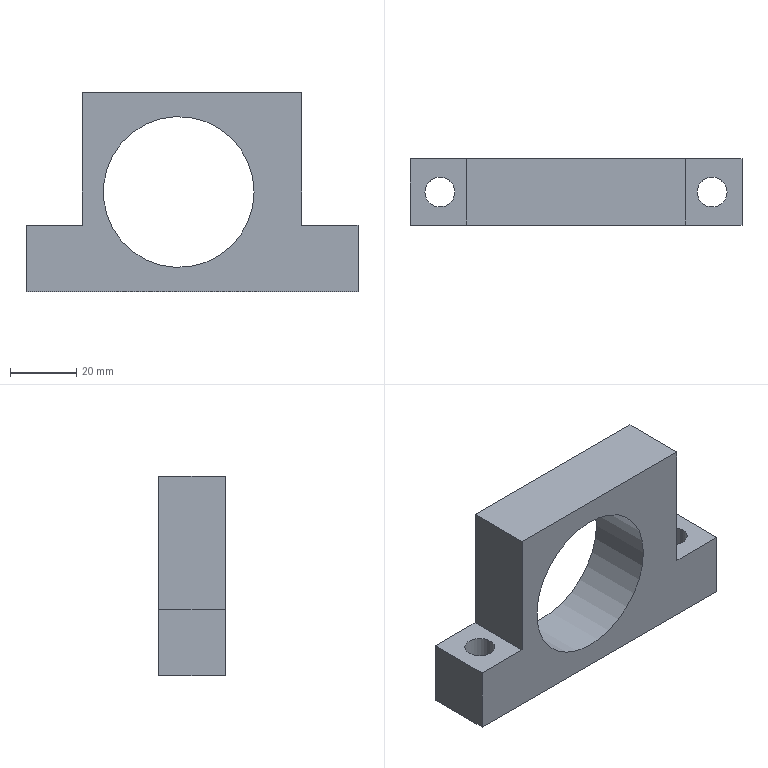Part | NX | features MAIN_BODY 2 | 1 solid | 13 faces | box 100 x 20 x 60 mm | volume 57879 mm3 | plane 10 | cylinder 3 | commonest cylinder face diameters 9 x2 45.4 x1
STEP:
#1=CARTESIAN_POINT('',(-575.,-600.,-225.));
#2=VERTEX_POINT('',#1);
#3=CARTESIAN_POINT('',(-575.,-620.,-225.));
#4=VERTEX_POINT('',#3);
#5=CARTESIAN_POINT('',(-575.,-565.,-225.));
#6=DIRECTION('',(0.,-1.,0.));
#7=VECTOR('',#6,1000.);
#8=LINE('',#5,#7);
#9=EDGE_CURVE('',#2,#4,#8,.T.);
#10=ORIENTED_EDGE('',*,*,#9,.F.);
#11=CARTESIAN_POINT('',(-575.,-600.,-245.));
#12=VERTEX_POINT('',#11);
#13=CARTESIAN_POINT('',(-575.,-600.,-245.));
#14=DIRECTION('',(0.,0.,1.));
#15=VECTOR('',#14,1000.);
#16=LINE('',#13,#15);
#17=EDGE_CURVE('',#12,#2,#16,.T.);
#18=ORIENTED_EDGE('',*,*,#17,.F.);
#19=CARTESIAN_POINT('',(-575.,-620.,-245.));
#20=VERTEX_POINT('',#19);
#21=CARTESIAN_POINT('',(-575.,-600.,-245.));
#22=DIRECTION('',(0.,-1.,0.));
#23=VECTOR('',#22,1000.);
#24=LINE('',#21,#23);
#25=EDGE_CURVE('',#12,#20,#24,.T.);
#26=ORIENTED_EDGE('',*,*,#25,.T.);
#27=CARTESIAN_POINT('',(-575.,-620.,-245.));
#28=DIRECTION('',(0.,0.,1.));
#29=VECTOR('',#28,1000.);
#30=LINE('',#27,#29);
#31=EDGE_CURVE('',#20,#4,#30,.T.);
#32=ORIENTED_EDGE('',*,*,#31,.T.);
#33=EDGE_LOOP('',(#10,#18,#26,#32));
#34=FACE_BOUND('',#33,.T.);
#35=CARTESIAN_POINT('',(-575.,-600.,-245.));
#36=DIRECTION('',(-1.,0.,0.));
#37=DIRECTION('',(0.,0.,-1.));
#38=AXIS2_PLACEMENT_3D('',#35,#36,#37);
#39=PLANE('',#38);
#40=ADVANCED_FACE('',(#34),#39,.T.);
#41=CARTESIAN_POINT('',(-492.,-600.,-185.));
#42=VERTEX_POINT('',#41);
#43=CARTESIAN_POINT('',(-492.,-620.,-185.));
#44=VERTEX_POINT('',#43);
#45=CARTESIAN_POINT('',(-492.,-565.,-185.));
#46=DIRECTION('',(0.,-1.,0.));
#47=VECTOR('',#46,1000.);
#48=LINE('',#45,#47);
#49=EDGE_CURVE('',#42,#44,#48,.T.);
#50=ORIENTED_EDGE('',*,*,#49,.F.);
#51=CARTESIAN_POINT('',(-558.,-600.,-185.));
#52=VERTEX_POINT('',#51);
#53=CARTESIAN_POINT('',(-575.,-600.,-185.));
#54=DIRECTION('',(1.,0.,0.));
#55=VECTOR('',#54,1000.);
#56=LINE('',#53,#55);
#57=EDGE_CURVE('',#52,#42,#56,.T.);
#58=ORIENTED_EDGE('',*,*,#57,.F.);
#59=CARTESIAN_POINT('',(-558.,-620.,-185.));
#60=VERTEX_POINT('',#59);
#61=CARTESIAN_POINT('',(-558.,-565.,-185.));
#62=DIRECTION('',(0.,-1.,0.));
#63=VECTOR('',#62,1000.);
#64=LINE('',#61,#63);
#65=EDGE_CURVE('',#52,#60,#64,.T.);
#66=ORIENTED_EDGE('',*,*,#65,.T.);
#67=CARTESIAN_POINT('',(-575.,-620.,-185.));
#68=DIRECTION('',(1.,0.,0.));
#69=VECTOR('',#68,1000.);
#70=LINE('',#67,#69);
#71=EDGE_CURVE('',#60,#44,#70,.T.);
#72=ORIENTED_EDGE('',*,*,#71,.T.);
#73=EDGE_LOOP('',(#50,#58,#66,#72));
#74=FACE_BOUND('',#73,.T.);
#75=CARTESIAN_POINT('',(-575.,-600.,-185.));
#76=DIRECTION('',(0.,0.,1.));
#77=DIRECTION('',(0.,1.,0.));
#78=AXIS2_PLACEMENT_3D('',#75,#76,#77);
#79=PLANE('',#78);
#80=ADVANCED_FACE('',(#74),#79,.T.);
#81=CARTESIAN_POINT('',(-475.,-600.,-225.));
#82=VERTEX_POINT('',#81);
#83=CARTESIAN_POINT('',(-475.,-620.,-225.));
#84=VERTEX_POINT('',#83);
#85=CARTESIAN_POINT('',(-475.,-565.,-225.));
#86=DIRECTION('',(0.,-1.,0.));
#87=VECTOR('',#86,1000.);
#88=LINE('',#85,#87);
#89=EDGE_CURVE('',#82,#84,#88,.T.);
#90=ORIENTED_EDGE('',*,*,#89,.T.);
#91=CARTESIAN_POINT('',(-475.,-620.,-245.));
#92=VERTEX_POINT('',#91);
#93=CARTESIAN_POINT('',(-475.,-620.,-185.));
#94=DIRECTION('',(0.,0.,-1.));
#95=VECTOR('',#94,1000.);
#96=LINE('',#93,#95);
#97=EDGE_CURVE('',#84,#92,#96,.T.);
#98=ORIENTED_EDGE('',*,*,#97,.T.);
#99=CARTESIAN_POINT('',(-475.,-600.,-245.));
#100=VERTEX_POINT('',#99);
#101=CARTESIAN_POINT('',(-475.,-600.,-245.));
#102=DIRECTION('',(0.,-1.,0.));
#103=VECTOR('',#102,1000.);
#104=LINE('',#101,#103);
#105=EDGE_CURVE('',#100,#92,#104,.T.);
#106=ORIENTED_EDGE('',*,*,#105,.F.);
#107=CARTESIAN_POINT('',(-475.,-600.,-185.));
#108=DIRECTION('',(0.,0.,-1.));
#109=VECTOR('',#108,1000.);
#110=LINE('',#107,#109);
#111=EDGE_CURVE('',#82,#100,#110,.T.);
#112=ORIENTED_EDGE('',*,*,#111,.F.);
#113=EDGE_LOOP('',(#90,#98,#106,#112));
#114=FACE_BOUND('',#113,.T.);
#115=CARTESIAN_POINT('',(-475.,-600.,-185.));
#116=DIRECTION('',(1.,0.,0.));
#117=DIRECTION('',(0.,0.,1.));
#118=AXIS2_PLACEMENT_3D('',#115,#116,#117);
#119=PLANE('',#118);
#120=ADVANCED_FACE('',(#114),#119,.T.);
#121=CARTESIAN_POINT('',(-479.5,-610.,-245.));
#122=VERTEX_POINT('',#121);
#123=CARTESIAN_POINT('',(-484.,-610.,-245.));
#124=DIRECTION('',(0.,0.,1.));
#125=DIRECTION('',(1.,0.,0.));
#126=AXIS2_PLACEMENT_3D('',#123,#124,#125);
#127=CIRCLE('',#126,4.5);
#128=EDGE_CURVE('',#122,#122,#127,.T.);
#129=ORIENTED_EDGE('',*,*,#128,.T.);
#130=EDGE_LOOP('',(#129));
#131=FACE_BOUND('',#130,.T.);
#132=CARTESIAN_POINT('',(-561.5,-610.,-245.));
#133=VERTEX_POINT('',#132);
#134=CARTESIAN_POINT('',(-566.,-610.,-245.));
#135=DIRECTION('',(0.,0.,1.));
#136=DIRECTION('',(1.,0.,0.));
#137=AXIS2_PLACEMENT_3D('',#134,#135,#136);
#138=CIRCLE('',#137,4.5);
#139=EDGE_CURVE('',#133,#133,#138,.T.);
#140=ORIENTED_EDGE('',*,*,#139,.T.);
#141=EDGE_LOOP('',(#140));
#142=FACE_BOUND('',#141,.T.);
#143=CARTESIAN_POINT('',(-475.,-620.,-245.));
#144=DIRECTION('',(-1.,0.,0.));
#145=VECTOR('',#144,1000.);
#146=LINE('',#143,#145);
#147=EDGE_CURVE('',#92,#20,#146,.T.);
#148=ORIENTED_EDGE('',*,*,#147,.T.);
#149=ORIENTED_EDGE('',*,*,#25,.F.);
#150=CARTESIAN_POINT('',(-475.,-600.,-245.));
#151=DIRECTION('',(-1.,0.,0.));
#152=VECTOR('',#151,1000.);
#153=LINE('',#150,#152);
#154=EDGE_CURVE('',#100,#12,#153,.T.);
#155=ORIENTED_EDGE('',*,*,#154,.F.);
#156=ORIENTED_EDGE('',*,*,#105,.T.);
#157=EDGE_LOOP('',(#148,#149,#155,#156));
#158=FACE_BOUND('',#157,.T.);
#159=CARTESIAN_POINT('',(-475.,-600.,-245.));
#160=DIRECTION('',(0.,0.,-1.));
#161=DIRECTION('',(1.,0.,0.));
#162=AXIS2_PLACEMENT_3D('',#159,#160,#161);
#163=PLANE('',#162);
#164=ADVANCED_FACE('',(#131,#142,#158),#163,.T.);
#165=CARTESIAN_POINT('',(-506.3,-600.,-215.));
#166=VERTEX_POINT('',#165);
#167=CARTESIAN_POINT('',(-529.,-600.,-215.));
#168=DIRECTION('',(0.,-1.,0.));
#169=DIRECTION('',(1.,0.,0.));
#170=AXIS2_PLACEMENT_3D('',#167,#168,#169);
#171=CIRCLE('',#170,22.7);
#172=EDGE_CURVE('',#166,#166,#171,.T.);
#173=ORIENTED_EDGE('',*,*,#172,.F.);
#174=EDGE_LOOP('',(#173));
#175=FACE_BOUND('',#174,.T.);
#176=CARTESIAN_POINT('',(-506.3,-620.,-215.));
#177=VERTEX_POINT('',#176);
#178=CARTESIAN_POINT('',(-529.,-620.,-215.));
#179=DIRECTION('',(0.,-1.,0.));
#180=DIRECTION('',(1.,0.,0.));
#181=AXIS2_PLACEMENT_3D('',#178,#179,#180);
#182=CIRCLE('',#181,22.7);
#183=EDGE_CURVE('',#177,#177,#182,.T.);
#184=ORIENTED_EDGE('',*,*,#183,.T.);
#185=EDGE_LOOP('',(#184));
#186=FACE_BOUND('',#185,.T.);
#187=CARTESIAN_POINT('',(-529.,-600.,-215.));
#188=DIRECTION('',(0.,-1.,0.));
#189=DIRECTION('',(-1.,0.,0.));
#190=AXIS2_PLACEMENT_3D('',#187,#188,#189);
#191=CYLINDRICAL_SURFACE('',#190,22.7);
#192=ADVANCED_FACE('',(#175,#186),#191,.F.);
#193=ORIENTED_EDGE('',*,*,#111,.T.);
#194=ORIENTED_EDGE('',*,*,#154,.T.);
#195=ORIENTED_EDGE('',*,*,#17,.T.);
#196=CARTESIAN_POINT('',(-558.,-600.,-225.));
#197=VERTEX_POINT('',#196);
#198=CARTESIAN_POINT('',(-575.,-600.,-225.));
#199=DIRECTION('',(-1.,0.,0.));
#200=VECTOR('',#199,1000.);
#201=LINE('',#198,#200);
#202=EDGE_CURVE('',#197,#2,#201,.T.);
#203=ORIENTED_EDGE('',*,*,#202,.F.);
#204=CARTESIAN_POINT('',(-558.,-600.,-185.));
#205=DIRECTION('',(0.,0.,-1.));
#206=VECTOR('',#205,1000.);
#207=LINE('',#204,#206);
#208=EDGE_CURVE('',#52,#197,#207,.T.);
#209=ORIENTED_EDGE('',*,*,#208,.F.);
#210=ORIENTED_EDGE('',*,*,#57,.T.);
#211=CARTESIAN_POINT('',(-492.,-600.,-225.));
#212=VERTEX_POINT('',#211);
#213=CARTESIAN_POINT('',(-492.,-600.,-185.));
#214=DIRECTION('',(0.,0.,1.));
#215=VECTOR('',#214,1000.);
#216=LINE('',#213,#215);
#217=EDGE_CURVE('',#212,#42,#216,.T.);
#218=ORIENTED_EDGE('',*,*,#217,.F.);
#219=CARTESIAN_POINT('',(-575.,-600.,-225.));
#220=DIRECTION('',(-1.,0.,0.));
#221=VECTOR('',#220,1000.);
#222=LINE('',#219,#221);
#223=EDGE_CURVE('',#82,#212,#222,.T.);
#224=ORIENTED_EDGE('',*,*,#223,.F.);
#225=EDGE_LOOP('',(#193,#194,#195,#203,#209,#210,#218,#224));
#226=FACE_BOUND('',#225,.T.);
#227=ORIENTED_EDGE('',*,*,#172,.T.);
#228=EDGE_LOOP('',(#227));
#229=FACE_BOUND('',#228,.T.);
#230=CARTESIAN_POINT('',(-575.,-600.,-185.));
#231=DIRECTION('',(0.,-1.,0.));
#232=DIRECTION('',(-1.,0.,0.));
#233=AXIS2_PLACEMENT_3D('',#230,#231,#232);
#234=PLANE('',#233);
#235=ADVANCED_FACE('',(#226,#229),#234,.F.);
#236=CARTESIAN_POINT('',(-492.,-620.,-225.));
#237=VERTEX_POINT('',#236);
#238=CARTESIAN_POINT('',(-575.,-620.,-225.));
#239=DIRECTION('',(-1.,0.,0.));
#240=VECTOR('',#239,1000.);
#241=LINE('',#238,#240);
#242=EDGE_CURVE('',#84,#237,#241,.T.);
#243=ORIENTED_EDGE('',*,*,#242,.T.);
#244=CARTESIAN_POINT('',(-492.,-620.,-185.));
#245=DIRECTION('',(0.,0.,1.));
#246=VECTOR('',#245,1000.);
#247=LINE('',#244,#246);
#248=EDGE_CURVE('',#237,#44,#247,.T.);
#249=ORIENTED_EDGE('',*,*,#248,.T.);
#250=ORIENTED_EDGE('',*,*,#71,.F.);
#251=CARTESIAN_POINT('',(-558.,-620.,-225.));
#252=VERTEX_POINT('',#251);
#253=CARTESIAN_POINT('',(-558.,-620.,-185.));
#254=DIRECTION('',(0.,0.,-1.));
#255=VECTOR('',#254,1000.);
#256=LINE('',#253,#255);
#257=EDGE_CURVE('',#60,#252,#256,.T.);
#258=ORIENTED_EDGE('',*,*,#257,.T.);
#259=CARTESIAN_POINT('',(-575.,-620.,-225.));
#260=DIRECTION('',(-1.,0.,0.));
#261=VECTOR('',#260,1000.);
#262=LINE('',#259,#261);
#263=EDGE_CURVE('',#252,#4,#262,.T.);
#264=ORIENTED_EDGE('',*,*,#263,.T.);
#265=ORIENTED_EDGE('',*,*,#31,.F.);
#266=ORIENTED_EDGE('',*,*,#147,.F.);
#267=ORIENTED_EDGE('',*,*,#97,.F.);
#268=EDGE_LOOP('',(#243,#249,#250,#258,#264,#265,#266,#267));
#269=FACE_BOUND('',#268,.T.);
#270=ORIENTED_EDGE('',*,*,#183,.F.);
#271=EDGE_LOOP('',(#270));
#272=FACE_BOUND('',#271,.T.);
#273=CARTESIAN_POINT('',(-575.,-620.,-185.));
#274=DIRECTION('',(0.,-1.,0.));
#275=DIRECTION('',(-1.,0.,0.));
#276=AXIS2_PLACEMENT_3D('',#273,#274,#275);
#277=PLANE('',#276);
#278=ADVANCED_FACE('',(#269,#272),#277,.T.);
#279=ORIENTED_EDGE('',*,*,#65,.F.);
#280=ORIENTED_EDGE('',*,*,#208,.T.);
#281=CARTESIAN_POINT('',(-558.,-565.,-225.));
#282=DIRECTION('',(0.,-1.,0.));
#283=VECTOR('',#282,1000.);
#284=LINE('',#281,#283);
#285=EDGE_CURVE('',#197,#252,#284,.T.);
#286=ORIENTED_EDGE('',*,*,#285,.T.);
#287=ORIENTED_EDGE('',*,*,#257,.F.);
#288=EDGE_LOOP('',(#279,#280,#286,#287));
#289=FACE_BOUND('',#288,.T.);
#290=CARTESIAN_POINT('',(-558.,-565.,-185.));
#291=DIRECTION('',(1.,0.,0.));
#292=DIRECTION('',(0.,0.,1.));
#293=AXIS2_PLACEMENT_3D('',#290,#291,#292);
#294=PLANE('',#293);
#295=ADVANCED_FACE('',(#289),#294,.F.);
#296=CARTESIAN_POINT('',(-561.5,-610.,-225.));
#297=VERTEX_POINT('',#296);
#298=CARTESIAN_POINT('',(-566.,-610.,-225.));
#299=DIRECTION('',(0.,0.,1.));
#300=DIRECTION('',(1.,0.,0.));
#301=AXIS2_PLACEMENT_3D('',#298,#299,#300);
#302=CIRCLE('',#301,4.5);
#303=EDGE_CURVE('',#297,#297,#302,.T.);
#304=ORIENTED_EDGE('',*,*,#303,.F.);
#305=EDGE_LOOP('',(#304));
#306=FACE_BOUND('',#305,.T.);
#307=ORIENTED_EDGE('',*,*,#285,.F.);
#308=ORIENTED_EDGE('',*,*,#202,.T.);
#309=ORIENTED_EDGE('',*,*,#9,.T.);
#310=ORIENTED_EDGE('',*,*,#263,.F.);
#311=EDGE_LOOP('',(#307,#308,#309,#310));
#312=FACE_BOUND('',#311,.T.);
#313=CARTESIAN_POINT('',(-558.,-565.,-225.));
#314=DIRECTION('',(0.,0.,-1.));
#315=DIRECTION('',(1.,0.,0.));
#316=AXIS2_PLACEMENT_3D('',#313,#314,#315);
#317=PLANE('',#316);
#318=ADVANCED_FACE('',(#306,#312),#317,.F.);
#319=CARTESIAN_POINT('',(-479.5,-610.,-225.));
#320=VERTEX_POINT('',#319);
#321=CARTESIAN_POINT('',(-484.,-610.,-225.));
#322=DIRECTION('',(0.,0.,1.));
#323=DIRECTION('',(1.,0.,0.));
#324=AXIS2_PLACEMENT_3D('',#321,#322,#323);
#325=CIRCLE('',#324,4.5);
#326=EDGE_CURVE('',#320,#320,#325,.T.);
#327=ORIENTED_EDGE('',*,*,#326,.F.);
#328=EDGE_LOOP('',(#327));
#329=FACE_BOUND('',#328,.T.);
#330=ORIENTED_EDGE('',*,*,#89,.F.);
#331=ORIENTED_EDGE('',*,*,#223,.T.);
#332=CARTESIAN_POINT('',(-492.,-565.,-225.));
#333=DIRECTION('',(0.,-1.,0.));
#334=VECTOR('',#333,1000.);
#335=LINE('',#332,#334);
#336=EDGE_CURVE('',#212,#237,#335,.T.);
#337=ORIENTED_EDGE('',*,*,#336,.T.);
#338=ORIENTED_EDGE('',*,*,#242,.F.);
#339=EDGE_LOOP('',(#330,#331,#337,#338));
#340=FACE_BOUND('',#339,.T.);
#341=CARTESIAN_POINT('',(-475.,-565.,-225.));
#342=DIRECTION('',(0.,0.,-1.));
#343=DIRECTION('',(1.,0.,0.));
#344=AXIS2_PLACEMENT_3D('',#341,#342,#343);
#345=PLANE('',#344);
#346=ADVANCED_FACE('',(#329,#340),#345,.F.);
#347=ORIENTED_EDGE('',*,*,#336,.F.);
#348=ORIENTED_EDGE('',*,*,#217,.T.);
#349=ORIENTED_EDGE('',*,*,#49,.T.);
#350=ORIENTED_EDGE('',*,*,#248,.F.);
#351=EDGE_LOOP('',(#347,#348,#349,#350));
#352=FACE_BOUND('',#351,.T.);
#353=CARTESIAN_POINT('',(-492.,-565.,-225.));
#354=DIRECTION('',(-1.,0.,0.));
#355=DIRECTION('',(0.,0.,-1.));
#356=AXIS2_PLACEMENT_3D('',#353,#354,#355);
#357=PLANE('',#356);
#358=ADVANCED_FACE('',(#352),#357,.F.);
#359=ORIENTED_EDGE('',*,*,#139,.F.);
#360=EDGE_LOOP('',(#359));
#361=FACE_BOUND('',#360,.T.);
#362=ORIENTED_EDGE('',*,*,#303,.T.);
#363=EDGE_LOOP('',(#362));
#364=FACE_BOUND('',#363,.T.);
#365=CARTESIAN_POINT('',(-566.,-610.,-255.));
#366=DIRECTION('',(0.,0.,1.));
#367=DIRECTION('',(0.,1.,0.));
#368=AXIS2_PLACEMENT_3D('',#365,#366,#367);
#369=CYLINDRICAL_SURFACE('',#368,4.5);
#370=ADVANCED_FACE('',(#361,#364),#369,.F.);
#371=ORIENTED_EDGE('',*,*,#128,.F.);
#372=EDGE_LOOP('',(#371));
#373=FACE_BOUND('',#372,.T.);
#374=ORIENTED_EDGE('',*,*,#326,.T.);
#375=EDGE_LOOP('',(#374));
#376=FACE_BOUND('',#375,.T.);
#377=CARTESIAN_POINT('',(-484.,-610.,-255.));
#378=DIRECTION('',(0.,0.,1.));
#379=DIRECTION('',(0.,1.,0.));
#380=AXIS2_PLACEMENT_3D('',#377,#378,#379);
#381=CYLINDRICAL_SURFACE('',#380,4.5);
#382=ADVANCED_FACE('',(#373,#376),#381,.F.);
#383=CLOSED_SHELL('',(#40,#80,#120,#164,#192,#235,#278,#295,#318,#346,#358,#370,#382));
#384=MANIFOLD_SOLID_BREP('',#383);
#385=(LENGTH_UNIT()NAMED_UNIT(*)SI_UNIT(.MILLI.,.METRE.));
#386=UNCERTAINTY_MEASURE_WITH_UNIT(LENGTH_MEASURE(0.00001),#385,'','');
#387=(NAMED_UNIT(*)PLANE_ANGLE_UNIT()SI_UNIT($,.RADIAN.));
#388=(NAMED_UNIT(*)SI_UNIT($,.STERADIAN.)SOLID_ANGLE_UNIT());
#389=(GEOMETRIC_REPRESENTATION_CONTEXT(3)GLOBAL_UNCERTAINTY_ASSIGNED_CONTEXT((#386))GLOBAL_UNIT_ASSIGNED_CONTEXT((#385,#387,#388))REPRESENTATION_CONTEXT('',''));
#390=ADVANCED_BREP_SHAPE_REPRESENTATION('',(#384),#389);